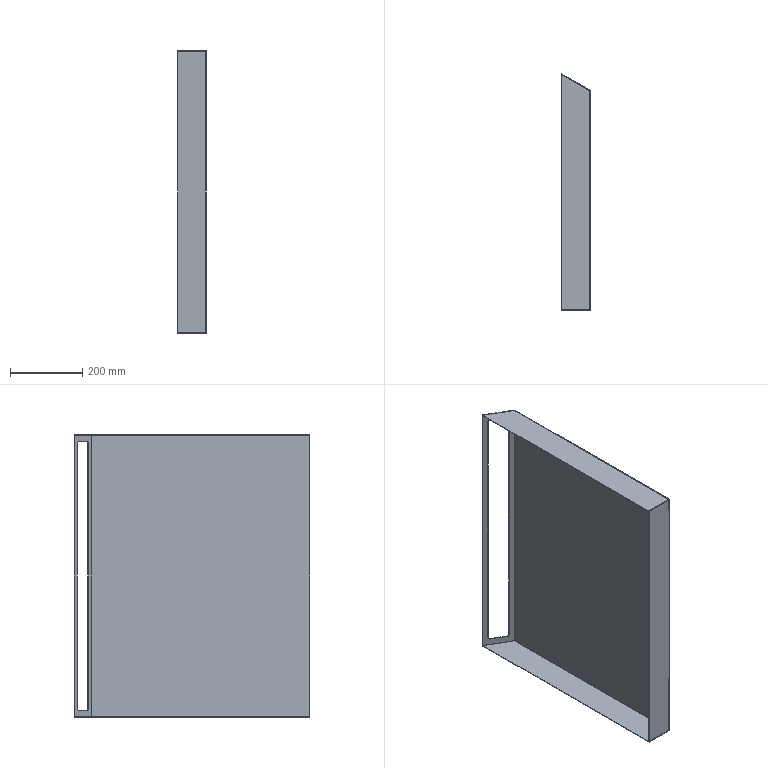Part | STEP file | Push button box_default<machined> | 3 solids | 42 faces | box 80 x 650.121 x 780 mm | volume 985013 mm3 | plane 34 | cylinder 8 | commonest cylinder face diameters 10 x4 0.2 x2 3.2 x2